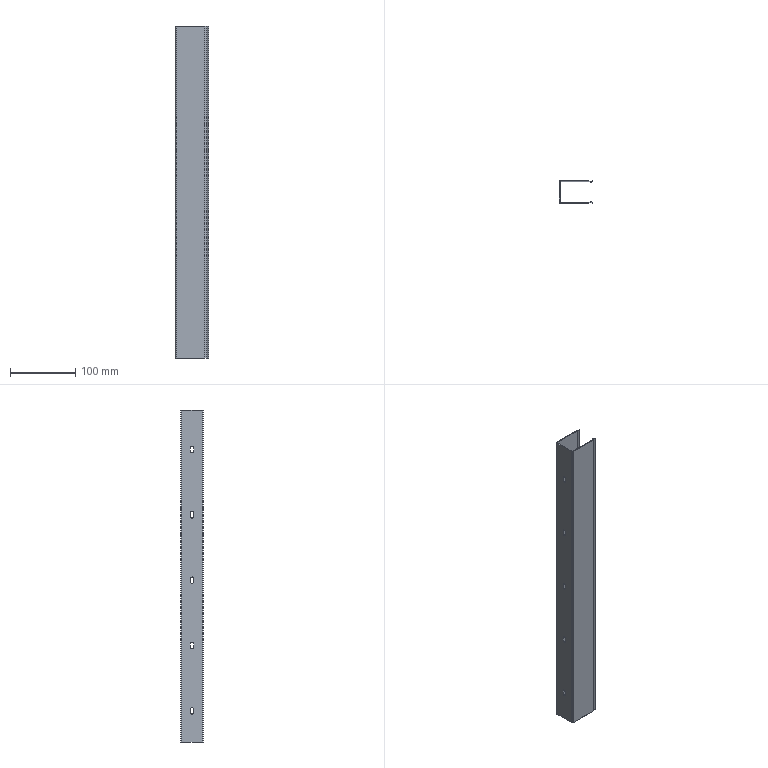Part | STEP file | 35 Cable Tray_508 | 1 solid | 47 faces | box 50.625 x 35 x 508 mm | volume 68787 mm3 | plane 28 | cylinder 19 | commonest cylinder face diameters 5 x15 1 x2 3 x2